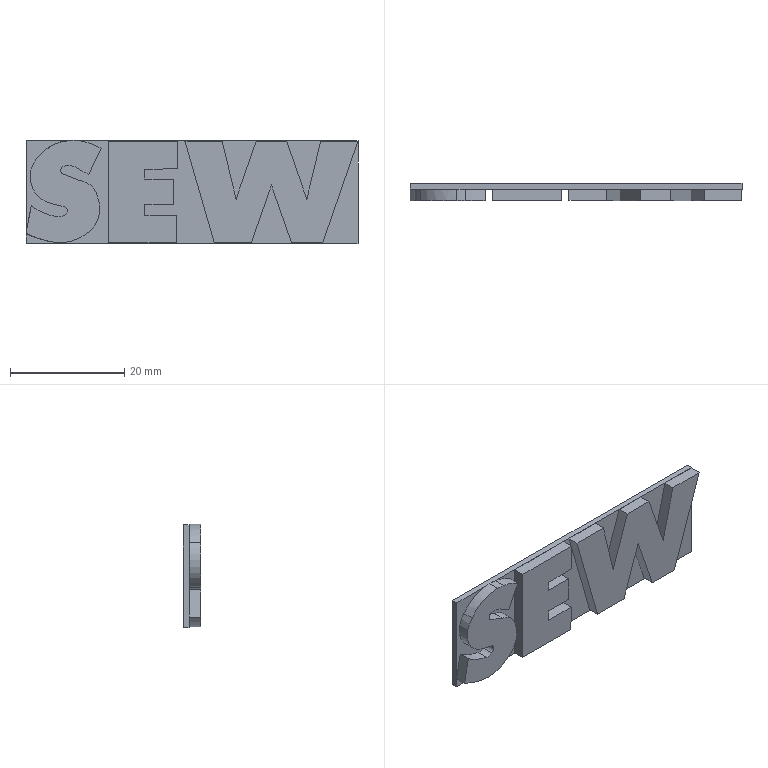Part | SolidWorks | features BaseBody 1 | 1 solid | 56 faces | box 58.086 x 3 x 18.091 mm | volume 2435 mm3 | plane 41 | cylinder 15 | commonest cylinder face diameters 5.974 x2 15.495 x2 1.626 x1 1.681 x1 4.595 x1 7.172 x1